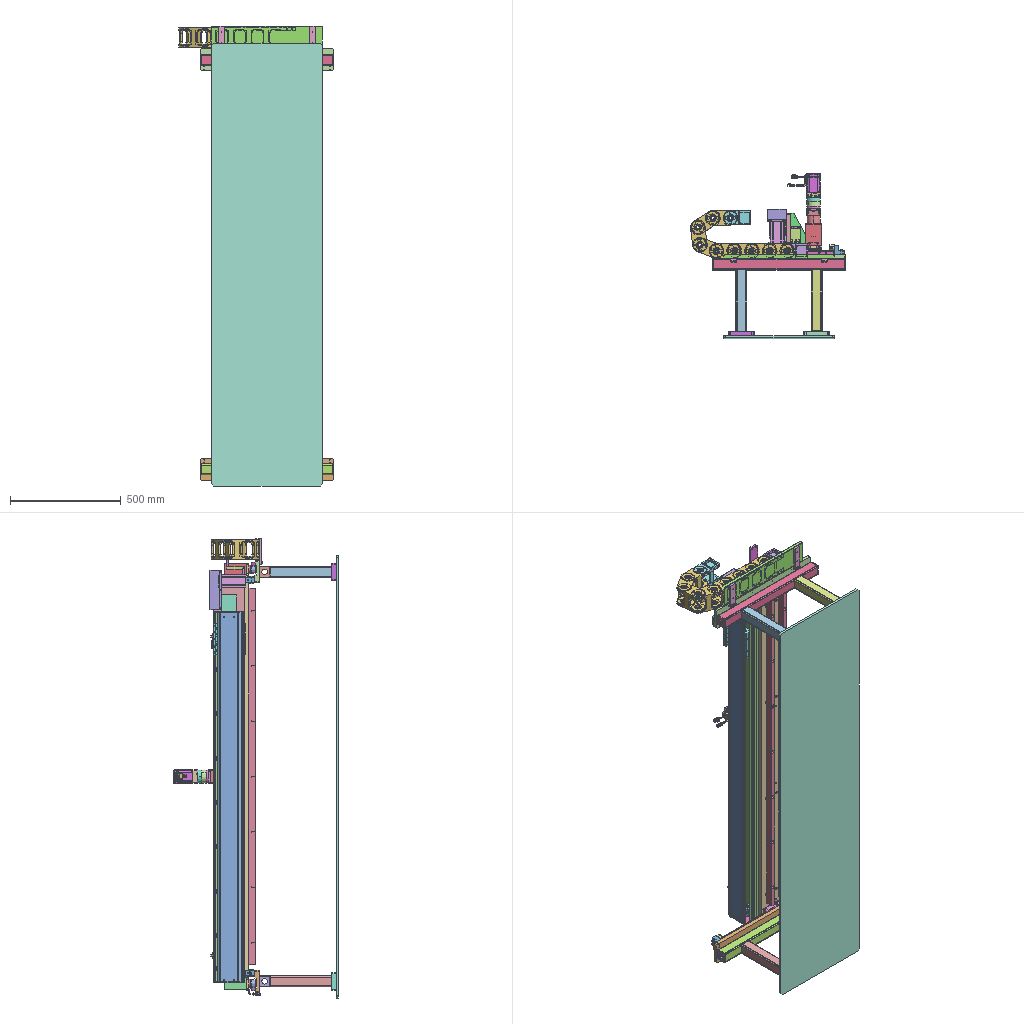Assembly | SolidWorks | 120 different items | 444 placed | box 699 x 745 x 2078 mm
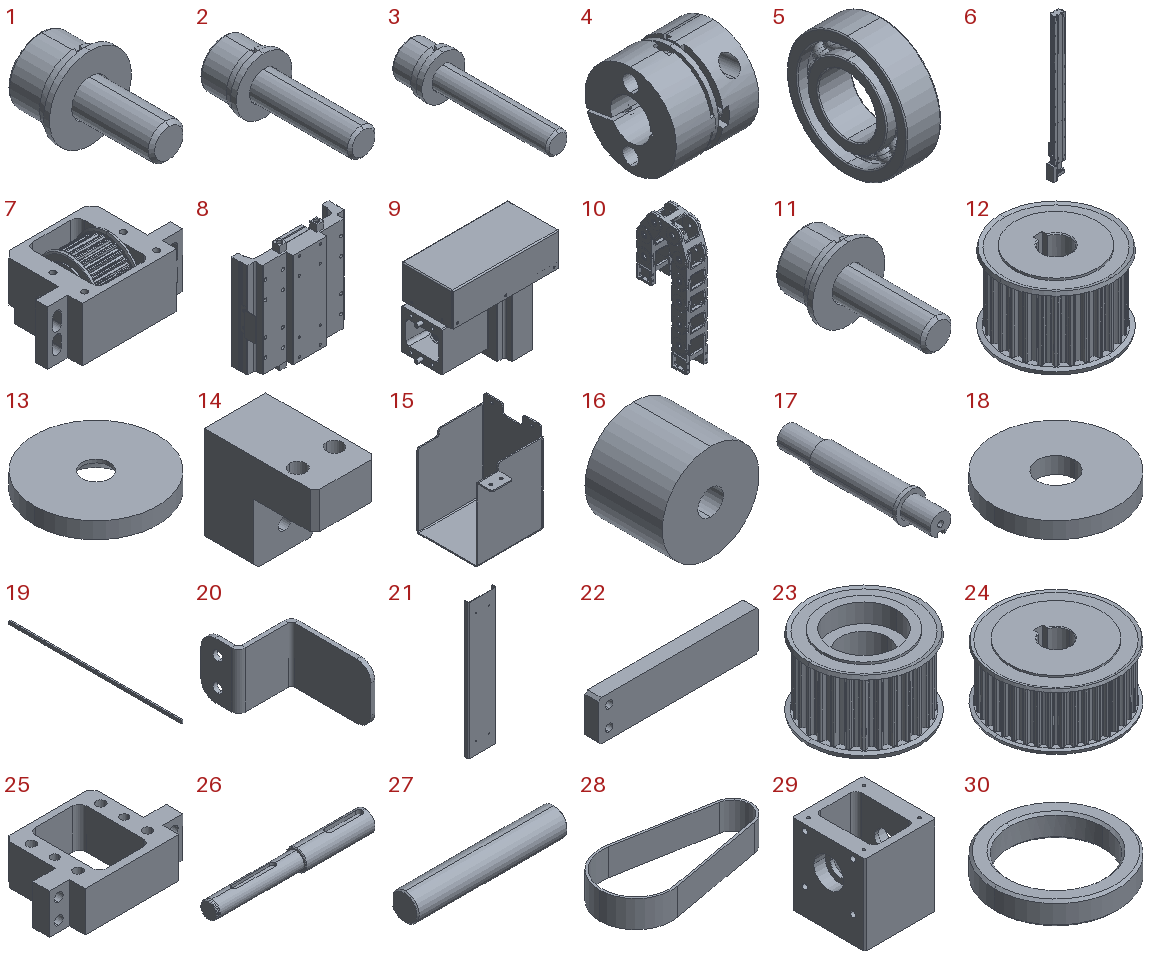Parts list (item | name | quantity | parent item | size | volume | features):
1 | (subassembly) | x2 | - | 7 x 11 x 7 mm | 152.048 mm3 | features RefAxis 1
2 | (subassembly) | x4 | - | 10 x 25 x 10 mm | 748.353 mm3 | features RefAxis 1
3 | (subassembly) | x12 | - | 12 x 41 x 12 mm | 1641 mm3 | features RefAxis 1
4 | (subassembly) | x2 | - | 29 x 32 x 32 mm | 15299 mm3 | -
5 | (subassembly) | x8 | - | 10 x 35 x 35 mm | 5427 mm3 | -
6 | (subassembly) | x1 | - | - | 6114333 mm3 | -
7 | (subassembly) | x1 | in 6 | 100 x 61 x 48 mm | 123898 mm3 | -
8 | (subassembly) | x2 | in 6 | 150 x 44 x 160 mm | 393138 mm3 | -
9 | (subassembly) | x1 | in 6 | 195.5 x 85 x 163 mm | 876200 mm3 | -
10 | (subassembly) | x1 | - | 93.598 x 215.392 x 529.568 mm | 1411050 mm3 | -
11 | (subassembly) | x4 | - | 7 x 13 x 7 mm | 166.185 mm3 | features RefAxis 1
12 | - | x1 | in 9 | 48 x 48 x 32 mm | 40101 mm3 | features BaseBody 1
13 | - | x2 | - | 15 x 15 x 2 mm | 317.309 mm3 | features Extrusion 1, HoleWzd 1
14 | - | x4 | - | 25 x 45 x 40 mm | 27816 mm3 | features Chamfer 2, HoleWzd 2, Extrusion 1, ICE 1
15 | - | x1 | - | 82.5 x 93.5 x 112 mm | 44800 mm3 | features EdgeFlange 2, HoleWzd 2, ICE 2, SMWeldBead 2, BreakCorner 1, FlatPattern 1, MoveFace 1, SMBaseFlange 1, SheetMetal 1
16 | - | x4 | - | 25 x 20 x 25 mm | 8476 mm3 | features Extrusion 1, HoleWzd 1
17 | - | x2 | - | 17 x 87.5 x 17 mm | 12724 mm3 | features ICE 3, HoleWzd 2, RefAxis 1, Revolution 1
18 | - | x4 | - | 15 x 15 x 2 mm | 321.621 mm3 | features Extrusion 1
19 | - | x2 | - | 18 x 1700 x 30 mm | 889358 mm3 | features Chamfer 1, Extrusion 1, HoleWzd 1
20 | - | x1 | - | 20.5 x 42 x 20 mm | 1726 mm3 | features BreakCorner 1, FlatPattern 1, HoleWzd 1, SMBaseFlange 1, SheetMetal 1
21 | - | x1 | - | 103 x 16.5 x 500 mm | 98465 mm3 | features BreakCorner 1, FlatPattern 1, HoleWzd 1, SMBaseFlange 1, SheetMetal 1
22 | - | x2 | - | 120 x 10 x 30 mm | 35369 mm3 | features HoleWzd 2, BreakCorner 1, FlatPattern 1, SMBaseFlange 1, SheetMetal 1
23 | - | x1 | in 7 | 48 x 48 x 32 mm | 29312 mm3 | features BaseBody 1
24 | - | x1 | in 9 | 67 x 67 x 32 mm | 86372 mm3 | features BaseBody 1
25 | - | x1 | in 6 | 100 x 63 x 30 mm | 67109 mm3 | features BaseBody 1
26 | - | x1 | in 9 | 114 x 15 x 15 mm | 15429 mm3 | features BaseBody 1
27 | - | x1 | in 7 | 66 x 12 x 12 mm | 7331 mm3 | features BaseBody 1
28 | - | x1 | in 9 | 140.79 x 66.7 x 25 mm | 16805 mm3 | features BaseBody 1
29 | - | x1 | in 9 | 66 x 68 x 75 mm | 164943 mm3 | features BaseBody 1
30 | - | x2 | in 7 | 16 x 16 x 3 mm | 250.27 mm3 | features BaseBody 1
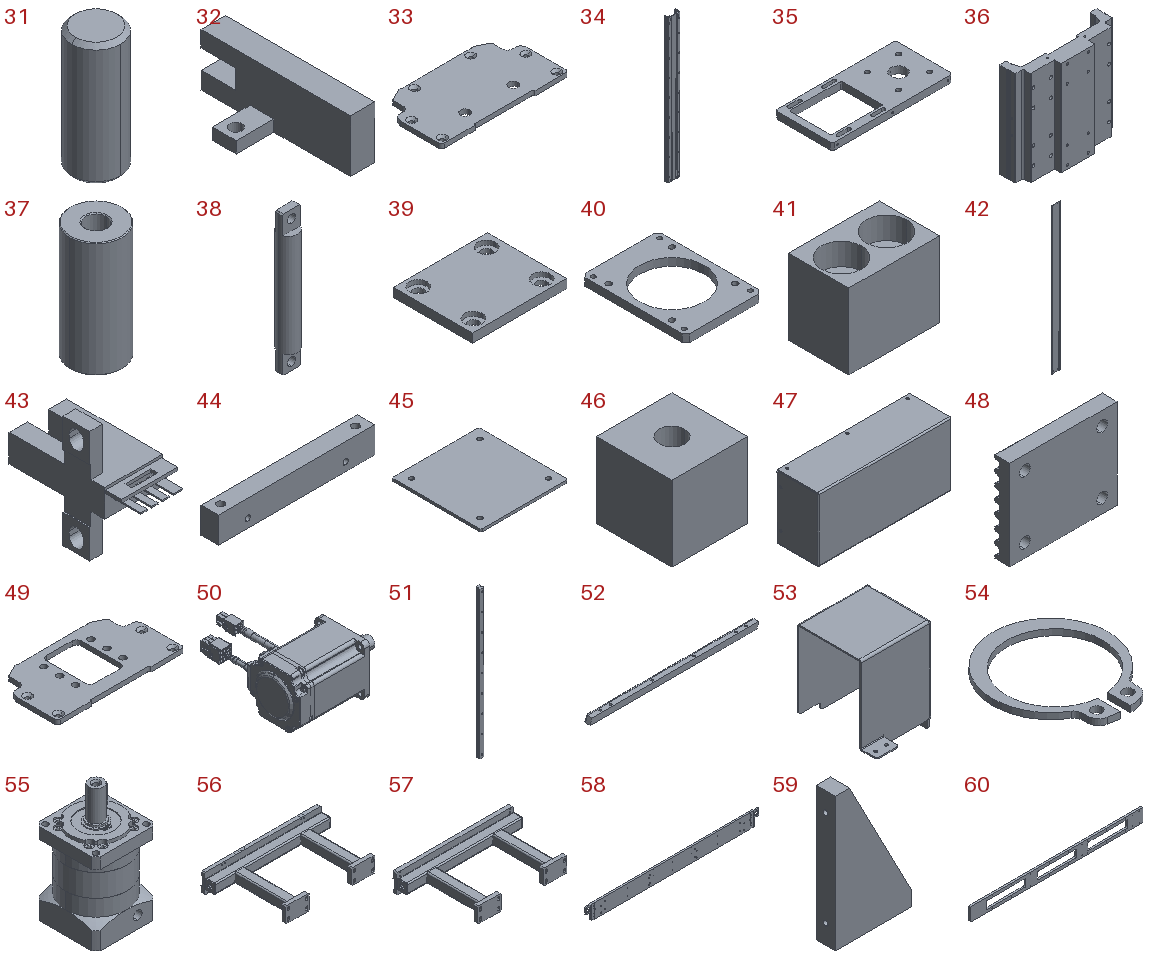31 | - | x2 | in 9 | 6 x 6 x 15 mm | 419.664 mm3 | features BaseBody 1
32 | - | x2 | in 6 | 26 x 39 x 13.7 mm | 3424 mm3 | features BaseBody 1
33 | - | x1 | in 6 | 140 x 76.005 x 5 mm | 46703 mm3 | features BaseBody 1
34 | - | x1 | in 6 | 140 x 53 x 1667 mm | 3998798 mm3 | features BaseBody 1
35 | - | x1 | in 9 | 175 x 83 x 10 mm | 88673 mm3 | features BaseBody 1
36 | - | x2 | in 8 | 144 x 44 x 140 mm | 348731 mm3 | features BaseBody 1
37 | - | x2 | in 8 | 20 x 20 x 44 mm | 11548 mm3 | features BaseBody 1
38 | - | x2 | in 8 | 8 x 8 x 60 mm | 2527 mm3 | features BaseBody 1
39 | - | x4 | in 8 | 43 x 36 x 4 mm | 5663 mm3 | features BaseBody 1
40 | - | x1 | in 9 | 60 x 82 x 6 mm | 17093 mm3 | features BaseBody 1
41 | - | x2 | in 6 | 18 x 12 x 15 mm | 2460 mm3 | features BaseBody 1
42 | - | x1 | in 6 | 109 x 8.5 x 1667 mm | 552829 mm3 | features BaseBody 1
43 | - | x3 | - | 13.7 x 28.4 x 26 mm | 1939 mm3 | features BaseBody 1
44 | - | x1 | in 6 | 72 x 8 x 12 mm | 6628 mm3 | features BaseBody 1
45 | - | x1 | in 9 | 66 x 68 x 2 mm | 8899 mm3 | features BaseBody 1
46 | - | x8 | in 8 | 10 x 10 x 10 mm | 827.255 mm3 | features BaseBody 1
47 | - | x1 | in 9 | 177 x 55 x 85 mm | 42380 mm3 | features BaseBody 1
48 | - | x4 | in 8 | 43 x 6 x 36 mm | 7398 mm3 | features BaseBody 1
49 | - | x1 | in 6 | 140 x 76.005 x 5 mm | 36774 mm3 | features BaseBody 1
50 | - | x1 | - | - | - | features RefSurface 19, BaseBody 5
51 | - | x1 | - | 15 x 15 x 500 mm | 91810 mm3 | features MirrorStock 1
52 | - | x1 | - | 506 x 17 x 17 mm | 126996 mm3 | features MirrorStock 1
53 | - | x1 | - | 82.5 x 93.5 x 112 mm | 44800 mm3 | features MirrorStock 1
54 | - | x8 | - | 18.95 x 21.754 x 1 mm | 100.896 mm3 | features Extrusion 1, Fillet 1
55 | - | x1 | - | 60 x 60 x 115 mm | 222679 mm3 | features BaseBody 7
56 | - | x1 | - | 600 x 368.308 x 100 mm | 1935248 mm3 | features HoleWzd 1, MirrorStock 1
57 | - | x1 | - | 600 x 368.308 x 100 mm | 1935957 mm3 | features HoleWzd 6, Chamfer 3, ICE 3, Cut 2, EndCap 1, MirrorPattern 1, WeldMemberFeat 1, WeldmentFeature 1
58 | - | x1 | - | 1924 x 20 x 160 mm | 5814736 mm3 | features HoleWzd 9, Cut 4, Chamfer 3, MirrorPattern 3, Fillet 2, Extrusion 1
59 | - | x4 | - | 80 x 20 x 140 mm | 141533 mm3 | features HoleWzd 2, Extrusion 1, ICE 1
60 | - | x1 | - | 1814 x 20 x 140 mm | 3064882 mm3 | features HoleWzd 3, Chamfer 1, Cut 1, Extrusion 1, Fillet 1
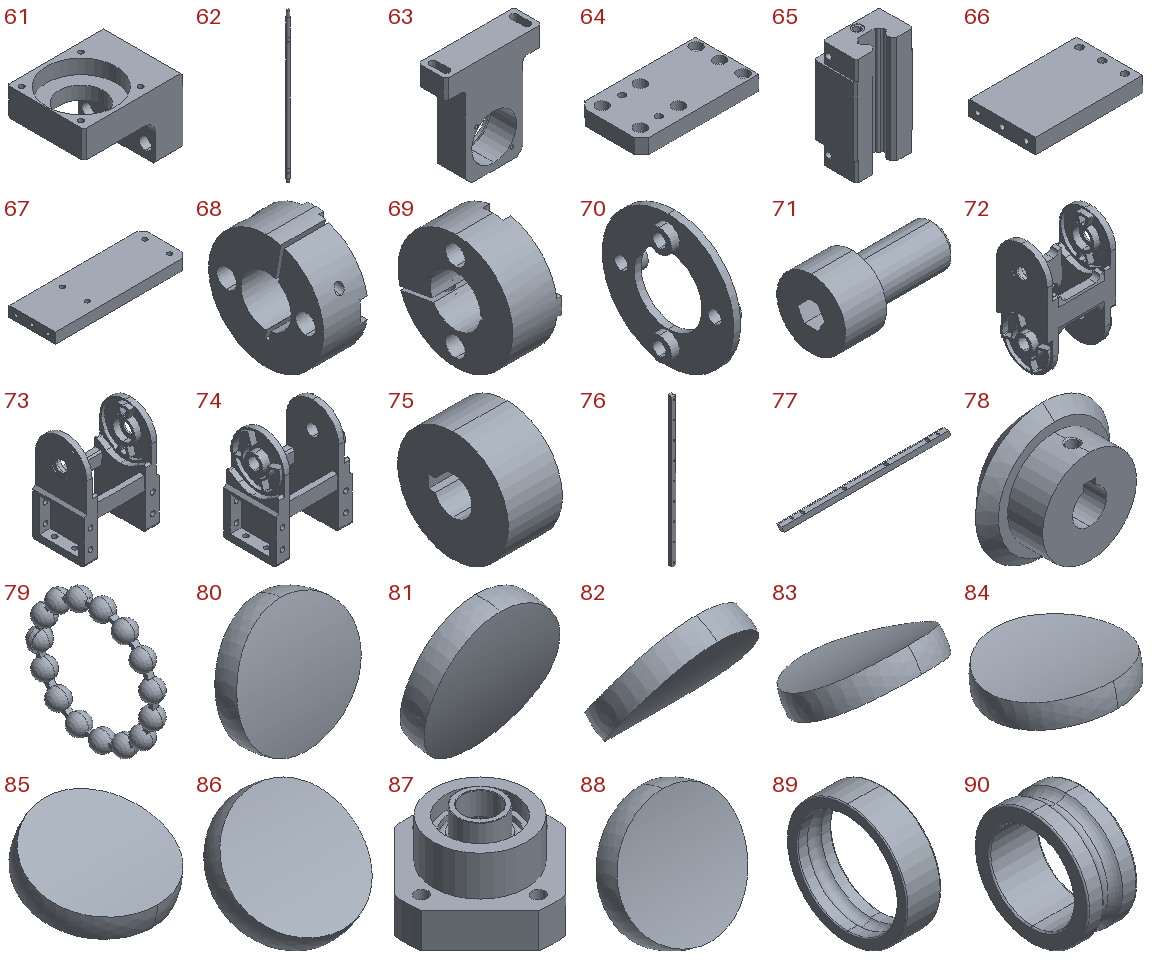61 | - | x2 | - | 90 x 70 x 60 mm | 158860 mm3 | features Cut 2, HoleWzd 2, Chamfer 1, Extrusion 1, Fillet 1
62 | - | x2 | - | 17 x 17 x 847.55 mm | 187223 mm3 | features ICE 7, Cut 1, Extrusion 1, HoleWzd 1, MoveFace 1
63 | - | x4 | - | 75 x 22 x 80 mm | 65225 mm3 | features ICE 3, Chamfer 2, HoleWzd 2, CirPattern 1, Extrusion 1, Fillet 1
64 | - | x1 | - | 80 x 43.6 x 10 mm | 31034 mm3 | features HoleWzd 3, Chamfer 1, Extrusion 1
65 | - | x4 | - | 34 x 23.7 x 61.4 mm | 36561 mm3 | features BaseBody 1
66 | - | x1 | - | 71 x 43.6 x 10 mm | 29737 mm3 | features HoleWzd 2, Extrusion 1
67 | - | x1 | - | 126 x 43.6 x 10 mm | 53864 mm3 | features HoleWzd 2, Chamfer 1, Extrusion 1
68 | - | x2 | in 4 | 13.7 x 32 x 32 mm | 6947 mm3 | features BaseBody 1
69 | - | x2 | in 4 | 13.7 x 32 x 32 mm | 6989 mm3 | features BaseBody 1
70 | - | x2 | in 4 | 5.6 x 31 x 31 mm | 974.208 mm3 | features BaseBody 1
71 | - | x8 | in 4 | 9 x 5 x 5 mm | 97.086 mm3 | features BaseBody 1
72 | - | x8 | in 10 | 89 x 65.39 x 145.39 mm | 145575 mm3 | features BaseBody 1
73 | - | x1 | in 10 | 93.538 x 64.35 x 124.74 mm | 121596 mm3 | features BaseBody 1
74 | - | x1 | in 10 | 93.598 x 64.35 x 124.74 mm | 124855 mm3 | features BaseBody 1
75 | - | x2 | - | 17 x 34.83 x 34.83 mm | 14145 mm3 | features BaseBody 1, ICE 1
76 | - | x1 | - | 15 x 15 x 500 mm | 91810 mm3 | features BaseBody 1, HoleWzd 1, ICE 1, MoveFace 1
77 | - | x1 | - | 506 x 17 x 17 mm | 126996 mm3 | features BaseBody 1
78 | - | x4 | - | 47.12 x 22.819 x 47.12 mm | 20583 mm3 | features 3DProfileFeature 1, BaseBody 1
79 | - | x8 | in 5 | 4.95 x 30.216 x 30.358 mm | 737.087 mm3 | features BaseBody 1
80 | - | x8 | in 5 | 4.95 x 1.888 x 4.932 mm | 17.147 mm3 | features BaseBody 1
81 | - | x8 | in 5 | 4.95 x 1.888 x 4.932 mm | 17.147 mm3 | features BaseBody 1
82 | - | x8 | in 5 | 4.95 x 3.576 x 4.449 mm | 17.147 mm3 | features BaseBody 1
83 | - | x8 | in 5 | 4.95 x 4.646 x 3.202 mm | 17.147 mm3 | features BaseBody 1
84 | - | x8 | in 5 | 4.95 x 4.95 x 1.444 mm | 17.147 mm3 | features BaseBody 1
85 | - | x8 | in 5 | 4.95 x 4.886 x 2.353 mm | 17.147 mm3 | features BaseBody 1
86 | - | x8 | in 5 | 4.95 x 4.203 x 3.911 mm | 17.147 mm3 | features BaseBody 1
87 | - | x2 | - | 63 x 63 x 46 mm | 51941 mm3 | features BaseBody 1
88 | - | x8 | in 5 | 4.95 x 2.793 x 4.793 mm | 17.147 mm3 | features BaseBody 1
89 | - | x8 | in 5 | 10 x 35 x 35 mm | 2757 mm3 | features BaseBody 1
90 | - | x8 | in 5 | 10 x 23 x 23 mm | 1693 mm3 | features BaseBody 1
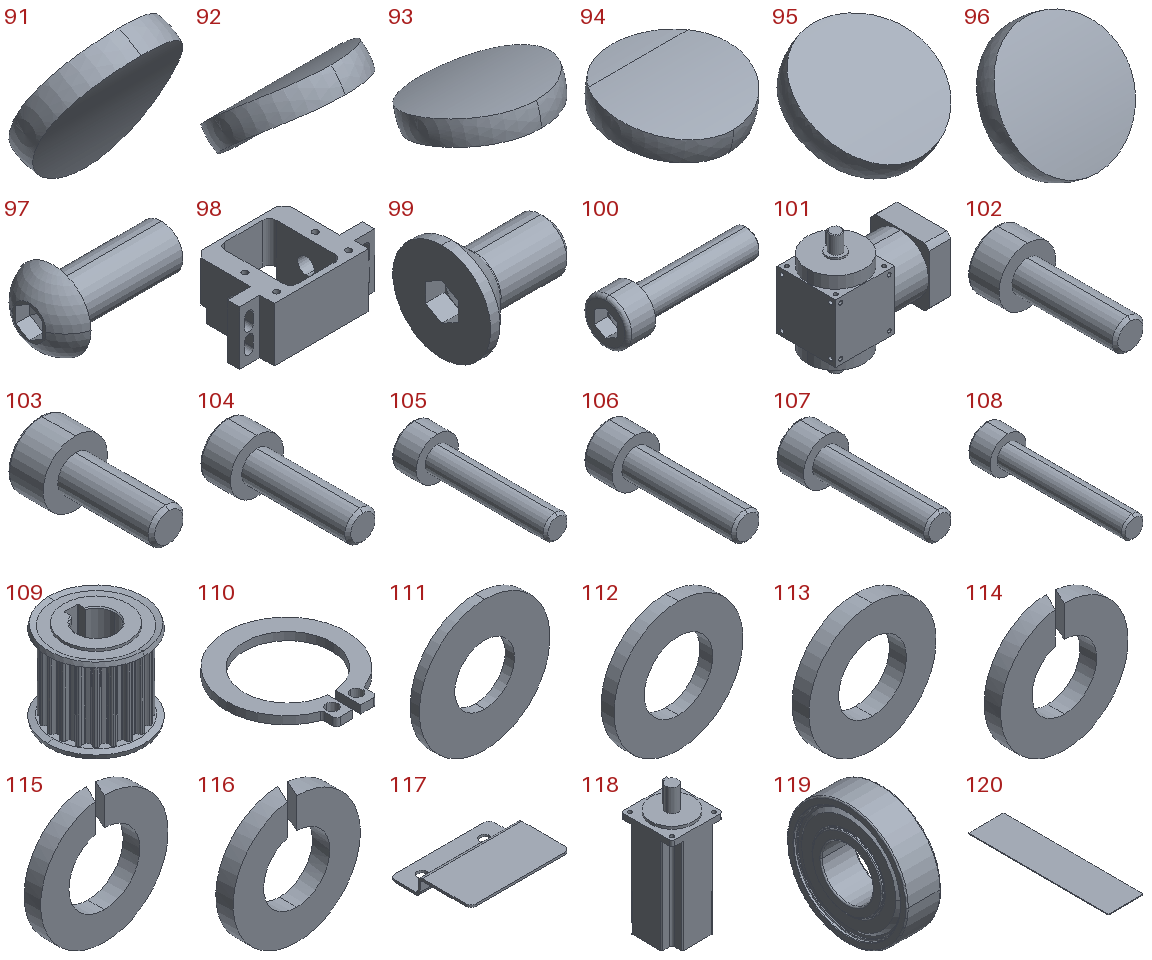91 | - | x8 | in 5 | 4.95 x 2.793 x 4.793 mm | 17.147 mm3 | features BaseBody 1
92 | - | x8 | in 5 | 4.95 x 4.203 x 3.911 mm | 17.147 mm3 | features BaseBody 1
93 | - | x8 | in 5 | 4.95 x 4.886 x 2.353 mm | 17.147 mm3 | features BaseBody 1
94 | - | x8 | in 5 | 4.95 x 4.95 x 1.444 mm | 17.148 mm3 | features BaseBody 1
95 | - | x8 | in 5 | 4.95 x 4.646 x 3.202 mm | 17.147 mm3 | features BaseBody 1
96 | - | x8 | in 5 | 4.95 x 3.576 x 4.449 mm | 17.147 mm3 | features BaseBody 1
97 | - | x8 | - | 48.8 x 28 x 28 mm | 11109 mm3 | features Cut 2, RevCut 2, Boss 1, Extrusion 1, Fillet 1, LPattern 1
98 | - | x1 | in 7 | 100 x 61 x 40 mm | 80408 mm3 | features BaseBody 1
99 | - | x2 | - | 8 x 7.53 x 7.53 mm | 138.584 mm3 | features RevCut 3, Chamfer 1, Cut 1, Fillet 1, LPattern 1, Revolution 1
100 | - | x4 | - | 31 x 10 x 10 mm | 1099 mm3 | features Fillet 2, RevCut 2, Boss 1, Chamfer 1, Cut 1, Extrusion 1, LPattern 1
101 | - | x1 | - | 128 x 65 x 134 mm | 554755 mm3 | features BaseBody 1
102 | - | x4 | in 11 | 5.5 x 13 x 5.5 mm | 134.154 mm3 | features ICE 2, Chamfer 1, Extrusion 1, Fillet 1, RefAxis 1
103 | - | x2 | in 1 | 5.5 x 11 x 5.5 mm | 120.016 mm3 | features ICE 2, Chamfer 1, Extrusion 1, Fillet 1, RefAxis 1
104 | - | x5 | - | 7 x 18 x 7 mm | 312.463 mm3 | features ICE 2, Chamfer 1, Extrusion 1, Fillet 1, RefAxis 1
105 | - | x18 | - | 7 x 24 x 7 mm | 387.861 mm3 | features ICE 2, Chamfer 1, Extrusion 1, Fillet 1, RefAxis 1
106 | - | x12 | in 2 | 8.5 x 25 x 8.5 mm | 639.095 mm3 | features ICE 2, Chamfer 1, Extrusion 1, Fillet 1, RefAxis 1
107 | - | x4 | - | 10 x 31 x 10 mm | 1108 mm3 | features ICE 2, Chamfer 1, Extrusion 1, Fillet 1, RefAxis 1
108 | - | x12 | in 3 | 10 x 41 x 10 mm | 1390 mm3 | features ICE 2, Chamfer 1, Extrusion 1, Fillet 1, RefAxis 1
109 | - | x1 | in 9 | 36 x 36 x 32 mm | 16182 mm3 | features BaseBody 1
110 | - | x1 | in 9 | 15.3 x 16.6 x 1 mm | 87.791 mm3 | features BaseBody 1
111 | - | x6 | in 1, 11 | 7 x 0.5 x 7 mm | 15.221 mm3 | features Extrusion 1, RefAxis 1
112 | - | x4 | in 2 | 10 x 1 x 10 mm | 56.478 mm3 | features Extrusion 1, RefAxis 1
113 | - | x12 | in 3 | 12 x 1.6 x 12 mm | 129.484 mm3 | features Extrusion 1, RefAxis 1
114 | - | x6 | in 1, 11 | 6.1 x 0.8 x 6.1 mm | 16.81 mm3 | features Extrusion 1, ICE 1, RefAxis 1
115 | - | x4 | in 2 | 9.15 x 1.2 x 9.15 mm | 52.779 mm3 | features Extrusion 1, ICE 1, RefAxis 1
116 | - | x12 | in 3 | 11.7 x 1.6 x 11.7 mm | 121.294 mm3 | features Extrusion 1, ICE 1, RefAxis 1
117 | - | x2 | in 8 | 35 x 28.6 x 6 mm | 900.941 mm3 | features BaseBody 1
118 | - | x1 | in 9 | 60 x 60 x 148 mm | 371098 mm3 | features BaseBody 1
119 | - | x4 | in 7, 9 | 8 x 28 x 28 mm | 3240 mm3 | features BaseBody 1
120 | - | x1 | - | 500 x 2000 x 10 mm | 9998000 mm3 | features Chamfer 1, Extrusion 1
Mates (type | each side: item.copy, entity, surface, feature):
In the top assembly
Coincident | 57.1 face plane Gb/6728-1986方形空心型钢 50 X 50 X 3(1) | 56.1 face plane
Coincident | 57.1 face plane Boss-Extrude 2 | 56.1 face plane
DistanceDim | 57.1 face plane Gb/6728-1986方形空心型钢 50 X 50 X 3(1) | 56.1 face plane
Coincident | 57.1 plane | assembly plane | 2 times
Symmetric | 57.1 face plane Gb/6728-1986方形空心型钢 50 X 50 X 3(1) | 56.1 face plane | assembly plane
Width | 76.1 face plane 输入1 | 76.1 face plane 输入1 | 57.1 face plane Boss-Extrude 2 | 57.1 face plane Boss-Extrude 2
DistanceDim | 76.1 plane | 57.1 face plane Boss-Extrude 2
Coincident | 65.1 face plane 输入1 | 76.1 face plane 输入1
Width | 65.1 face plane 输入1 | 65.1 face plane 输入1 | 76.1 face plane 输入1 | 76.1 face plane 输入1
Coincident | 76.1 face plane 输入1 | 65.2 face plane 输入1
Coincident | 65.1 face plane 输入1 | 65.2 face plane 输入1
DistanceDim | 65.2 face plane 输入1 | 65.1 face plane 输入1
Width | 65.2 face plane 输入1 | 65.1 face plane 输入1 | 58.1 face plane Boss-Extrude 1 | 58.1 face plane Boss-Extrude 1
Width | 57.1 face plane Gb/6728-1986方形空心型钢 50 X 50 X 3(1) | 56.1 face plane | 58.1 face plane Boss-Extrude 1 | 58.1 face plane Boss-Extrude 1
Width | 57.1 face plane Boss-Extrude 2 | 57.1 face plane Boss-Extrude 2 | 77.1 plane | 77.1 plane
Coincident | 58.1 face plane Boss-Extrude 1 | 60.1 face plane Boss-Extrude 1 | 2 times
Width | 60.1 face plane Boss-Extrude 1 | 60.1 face plane Boss-Extrude 1 | 58.1 face plane Boss-Extrude 1 | 58.1 face plane Boss-Extrude 1
Coincident | 60.1 face plane Boss-Extrude 1 | 34.1 face plane 输入1 | 2 times
Width | 60.1 face plane Boss-Extrude 1 | 60.1 face plane Boss-Extrude 1 | 33.1 face plane 输入1 | 47.1 face plane 输入1
Coincident | 101.1 face plane 输入1 | 55.1 face plane PRF60 Upper蓋版_D1-70 D2-5.5 D3-14 D4-17 D5-50 L1-30 L2-35 L3-3 A1-60 S1-3 S2-20 S3-5 S4-18 B-5 H-16 C-M5 标准-1-solid1
Concentric | 101.1 face cylinder 输入1 | 55.1 face cylinder PRF60 Upper蓋版_D1-70 D2-5.5 D3-14 D4-17 D5-50 L1-30 L2-35 L3-3 A1-60 S1-3 S2-20 S3-5 S4-18 B-5 H-16 C-M5 标准-1-solid1
Concentric | 50.1 face cylinder DEFAULT-1/DEFAULT-1-surface1 | 55.1 face cylinder PRF60 Lower蓋版_D6-60 D7-14 标准-1-solid1
Parallel | 50.1 face plane DEFAULT-1/DEFAULT-1-surface2 | 55.1 face plane PRF60-連接Plate-标准_D8-50 D9-70 D10-M10 L4-22 L6-32(22+10) L7-4 A2-60 R-39.5 标准-1-solid1
Coincident | 50.1 face plane DEFAULT-1/DEFAULT-1-surface2 | 55.1 face plane PRF60-連接Plate-标准_D8-50 D9-70 D10-M10 L4-22 L6-32(22+10) L7-4 A2-60 R-39.5 标准-1-solid1
Parallel | 101.1 face plane 输入1 | 55.1 face plane PRF60 Upper蓋版_D1-70 D2-5.5 D3-14 D4-17 D5-50 L1-30 L2-35 L3-3 A1-60 S1-3 S2-20 S3-5 S4-18 B-5 H-16 C-M5 标准-1-solid1
Parallel | 60.1 face plane Boss-Extrude 1 | 101.1 face plane 输入1
Width | 60.1 face plane Boss-Extrude 1 | 60.1 face plane Boss-Extrude 1 | 101.1 face plane 输入1 | 101.1 face plane 输入1
Coincident | 58.1 face plane Boss-Extrude 1 | 61.1 face plane Boss-Extrude 1
Width | 61.1 face plane Boss-Extrude 1 | 61.1 face plane Boss-Extrude 1 | 101.1 face plane 输入1 | 101.1 face plane 输入1
Coincident | 101.1 face plane 输入1 | 61.1 face plane Boss-Extrude 1
Coincident | 58.1 face plane Boss-Extrude 1 | 61.2 face plane Boss-Extrude 1
Coincident | 61.1 face plane Boss-Extrude 1 | 61.2 face plane Boss-Extrude 1
Coincident | 101.1 face plane 输入1 | 61.2 face plane Boss-Extrude 1
Concentric | 101.1 face cylinder 输入1 | 69.1 face cylinder 输入1
Concentric | 69.1 face cylinder 输入1 | 62.1 face cylinder Boss-Extrude 1
Coincident | 101.1 face plane 输入1 | 69.1 face plane 输入1
Coincident | 68.1 face plane 输入1 | 62.1 face plane Boss-Extrude 1
Concentric | 62.1 face cylinder Boss-Extrude 2 | 90.1 face cylinder 输入1
Concentric | 62.1 face cylinder Boss-Extrude 2 | 63.1 face cylinder Cut-Extrude 3
Parallel | 58.1 face plane Boss-Extrude 1 | 63.1 face plane Boss-Extrude 1
Coincident | 89.1 face plane 输入1 | 63.1 face plane Boss-Extrude 3
Concentric | 62.1 face cylinder Boss-Extrude 2 | 90.2 face cylinder 输入1
Coincident | 63.1 face plane Boss-Extrude 1 | 89.2 face plane 输入1
Coincident | 63.2 face plane Boss-Extrude 1 | 89.3 face plane 输入1
Concentric | 63.2 face cylinder Cut-Extrude 3 | 90.3 face cylinder 输入1
Concentric | 90.4 face cylinder 输入1 | 90.3 face cylinder 输入1
Coincident | 58.1 face plane Boss-Extrude 1 | 63.2 face plane Boss-Extrude 1
Coincident | 89.4 face plane 输入1 | 89.3 face plane 输入1
Coincident | 63.1 face plane Boss-Extrude 1 | 63.2 face plane Boss-Extrude 1
DistanceDim | 63.1 face plane Boss-Extrude 1 | 58.1 face plane Boss-Extrude 1
Coincident | 58.1 face plane Boss-Extrude 1 | 63.1 face plane Boss-Extrude 2
Concentric | 62.1 face cylinder Cut-Extrude 1 | 78.1 face cylinder 输入1
Coincident | 62.1 face plane Boss-Extrude 2 | 78.1 face plane 输入1
Coincident | 78.1 select_type:25 | 78.2 select_type:25
Parallel | 58.1 face plane Boss-Extrude 1 | 78.2 face plane 输入1
GearDim | 78.1 edge | 78.2 edge
Concentric | 101.1 face cylinder 输入1 | 61.2 face cylinder Cut-Extrude 2
Concentric | 78.2 face cylinder 输入1 | 17.1 face cylinder Revolve 1
Coincident | 78.2 face plane 输入1 | 17.1 face plane Revolve 1
Concentric | 17.1 face cylinder Revolve 1 | 87.1 face cylinder 输入1
Parallel | 58.1 face plane Boss-Extrude 1 | 87.1 face plane 输入1
Coincident | 58.1 face plane Cut-Extrude 1 | 87.1 face plane 输入1
Coincident | 57.1 face plane Boss-Extrude 2 | 76.1 face plane 输入1
Coincident | 57.1 face plane Cut-Extrude 2 | 77.1 face plane 输入1
DistanceDim | 17.1 axis | 77.1 face plane 输入1
Concentric | 17.1 face cylinder Boss-Extrude 1 | 75.1 face cylinder 输入1 | 2 times
Coincident | 17.1 face plane Revolve 1 | 75.1 face plane 输入1
DistanceDim | 58.1 face plane Boss-Extrude 1 | 65.1 face plane 输入1
Coincident | 62.1 face plane Cut-Extrude 11 | 78.1 face plane 输入1
Coincident | 78.2 face plane 输入1 | 17.1 face plane Cut-Extrude 1
Coincident | 58.1 face plane Boss-Extrude 1 | 59.1 face plane Boss-Extrude 1
Coincident | 59.1 face plane Boss-Extrude 1 | 60.1 face plane Boss-Extrude 1
Coincident | 58.1 face plane Boss-Extrude 1 | 59.2 face plane Boss-Extrude 1
Coincident | 60.1 face plane Boss-Extrude 1 | 59.2 face plane Boss-Extrude 1
DistanceDim | 60.1 face plane Boss-Extrude 1 | 59.1 face plane Boss-Extrude 1
DistanceDim | 59.2 face plane Boss-Extrude 1 | 60.1 face plane Boss-Extrude 1
Concentric | 17.1 face cylinder M4 Tapped Hole 2 | 18.1 face cylinder Boss-Extrude 1
Concentric | 18.1 face cylinder Boss-Extrude 1 | 100.1 face cylinder BaseBody
Coincident | 18.1 face plane Boss-Extrude 1 | 100.1 face plane BaseHead
Concentric | 75.1 face cylinder 输入1 | 13.1 face cylinder Boss-Extrude 1
Coincident | 17.1 face plane Boss-Extrude 1 | 13.1 face plane Boss-Extrude 1
Concentric | 13.1 face cylinder M3 开槽沉头木Screw的锥形沉头Hole 1 | 99.1 face cylinder Base
DistanceDim | 63.2 face plane Boss-Extrude 1 | 58.1 face plane Cut-Extrude 1
Width | 19.1 face plane Boss-Extrude 1 | 19.1 face plane Boss-Extrude 1 | 58.1 face plane Cut-Extrude 1 | 58.1 face plane Mirror 1
DistanceDim | 58.1 face plane Boss-Extrude 1 | 19.1 face plane Boss-Extrude 1
Coincident | 78.2 face plane 输入1 | 18.1 face plane Boss-Extrude 1
Coincident | 13.1 face cone M3 开槽沉头木Screw的锥形沉头Hole 1 | 99.1 face cone Base
Coincident | 58.1 face plane Boss-Extrude 1 | 19.1 face plane Boss-Extrude 1
Coincident | 58.1 face plane Boss-Extrude 1 | 19.2 face plane Boss-Extrude 1
Width | 19.1 face plane Boss-Extrude 1 | 19.2 face plane Boss-Extrude 1 | 58.1 face plane Boss-Extrude 1 | 58.1 face plane Boss-Extrude 1
Coincident | 19.1 face plane Boss-Extrude 1 | 19.2 face plane Boss-Extrude 1
Coincident | 57.1 face plane Boss-Extrude 2 | 14.1 face plane Boss-Extrude 1
Width | 14.1 face plane Boss-Extrude 1 | 14.1 face plane Boss-Extrude 1 | 76.1 face plane 输入1 | 76.1 face plane 输入1
Coincident | 76.1 face plane 输入1 | 14.1 face plane Boss-Extrude 1
Concentric | 14.1 face cylinder M6 Tapped Hole 1 | 16.1 face cylinder M6 六角圆柱头Screw的柱形沉头Hole 1
Coincident | 14.1 face plane Boss-Extrude 1 | 16.1 face plane Boss-Extrude 1
Coincident | 57.1 face plane Boss-Extrude 2 | 43.1 face plane 输入1
Width | 57.1 face plane Cut-Extrude 2 | 57.1 face plane Boss-Extrude 2 | 43.1 face plane 输入1 | 43.1 face plane 输入1
Coincident | 57.1 face plane Boss-Extrude 2 | 43.2 face plane 输入1
Width | 57.1 face plane Cut-Extrude 2 | 57.1 face plane Boss-Extrude 2 | 43.2 face plane 输入1 | 43.2 face plane 输入1
DistanceDim | 57.1 face plane Boss-Extrude 2 | 43.2 face plane 输入1
Coincident | 43.2 face plane 输入1 | 43.3 face plane 输入1 | 2 times
DistanceDim | 43.3 face plane 输入1 | 43.2 face plane 输入1
Coincident | 58.1 face plane Boss-Extrude 1 | 20.1 face plane Base-Flange 1
Width | 58.1 face plane Boss-Extrude 1 | 58.1 face plane Cut-Extrude 5 | 20.1 face plane Base-Flange 1 | 20.1 face plane Base-Flange 1
Coincident | 58.1 face plane Cut-Extrude 1 | 20.1 face plane Base-Flange 1
Concentric | 62.1 face cylinder M4 Tapped Hole 1 | 18.2 face cylinder Boss-Extrude 1
Coincident | 62.1 face plane Cut-Extrude 2 | 18.2 face plane Boss-Extrude 1
Concentric | 62.1 face cylinder M4 Tapped Hole 1 | 100.2 face cylinder BaseBody
Coincident | 100.2 face plane BaseHead | 18.2 face plane Boss-Extrude 1
Concentric | 63.2 face cylinder M3 Tapped Hole 1 | 97.1 face cylinder BaseBody
Coincident | 63.2 face plane Boss-Extrude 1 | 97.1 face plane BaseHead
Concentric | 63.2 face cylinder CirPattern 1 | 97.2 face cylinder BaseBody
Coincident | 63.2 face plane Boss-Extrude 1 | 97.2 face plane BaseHead
Concentric | 63.1 face cylinder M3 Tapped Hole 1 | 97.3 face cylinder BaseBody
Coincident | 63.1 face plane Boss-Extrude 1 | 97.3 face plane BaseHead
Concentric | 63.1 face cylinder CirPattern 1 | 97.4 face cylinder BaseBody
Coincident | 63.1 face plane Boss-Extrude 1 | 97.4 face plane BaseHead
Concentric | 62.1 face cylinder Cut-Extrude 15 | 54.1 face cylinder Boss-Extrude 1
Coincident | 90.3 face plane 输入1 | 54.1 face plane Boss-Extrude 1
Concentric | 62.1 face cylinder Cut-Extrude 14 | 54.2 face cylinder Boss-Extrude 1
Coincident | 90.4 face plane 输入1 | 54.2 face plane Boss-Extrude 1
Concentric | 62.1 face cylinder Cut-Extrude 13 | 54.3 face cylinder Boss-Extrude 1
Coincident | 90.1 face plane 输入1 | 54.3 face plane Boss-Extrude 1
Concentric | 62.1 face cylinder Cut-Extrude 12 | 54.4 face cylinder Boss-Extrude 1
Coincident | 90.2 face plane 输入1 | 54.4 face plane Boss-Extrude 1
Width | 21.1 face plane Base-Flange 1 | 21.1 face plane Base-Flange 1 | 56.1 face plane | 56.1 face plane
Coincident | 56.1 face plane | 21.1 face plane Base-Flange 1 | 2 times
Coincident | 56.1 face plane | 22.1 face plane Base-Flange 1
Coincident | 21.1 face plane Base-Flange 1 | 22.1 face plane Base-Flange 1
Coincident | 21.1 face plane Base-Flange 1 | 72.1 face plane 输入1
Width | 21.1 face plane Base-Flange 1 | 21.1 face plane Base-Flange 1 | 74.1 face plane 输入1 | 74.1 face plane 输入1
DistanceDim | 74.1 face plane 输入1 | 21.1 face plane Base-Flange 1
Coincident | 56.1 face plane | 22.2 face plane Base-Flange 1
Coincident | 21.1 face plane Base-Flange 1 | 22.2 face plane Base-Flange 1
Width | 21.1 face plane Base-Flange 1 | 21.1 face plane Base-Flange 1 | 22.2 face plane Base-Flange 1 | 22.1 face plane Base-Flange 1
LimitDistanceDim | 58.1 face plane Boss-Extrude 1 | 16.2 face plane Boss-Extrude 1
Coincident | 58.1 face plane Cut-Extrude 1 | 15.1 face plane Edge-Flange 1
Width | 87.1 face plane 输入1 | 87.1 face plane 输入1 | 15.1 face plane Edge-Flange 1 | 15.1 face plane Edge-Flange 1
Coincident | 58.1 face plane Boss-Extrude 1 | 15.1 face plane Edge-Flange 1
Coincident | 58.1 face plane Boss-Extrude 1 | 64.1 face plane Boss-Extrude 1
Symmetric | 65.3 plane | 64.1 face plane Boss-Extrude 1 | 64.1 face plane Boss-Extrude 1
DistanceDim | 64.1 face plane Boss-Extrude 1 | 58.1 face plane Mirror 1
Coincident | 64.1 face plane Boss-Extrude 1 | 66.1 face plane Boss-Extrude 1 | 4 times
Coincident | 66.1 face plane Boss-Extrude 1 | 67.1 face plane Boss-Extrude 1 | 3 times
DistanceDim | 22.2 face plane Base-Flange 1 | 21.1 face plane Base-Flange 1
Coincident | 57.1 face plane Boss-Extrude 3 | 120.1 face plane Boss-Extrude 1
Width | 120.1 face plane Boss-Extrude 1 | 120.1 face plane Boss-Extrude 1 | 57.1 face plane Boss-Extrude 3 | 57.1 face plane Boss-Extrude 3
Width | 120.1 face plane Boss-Extrude 1 | 120.1 face plane Boss-Extrude 1 | 57.1 face plane Boss-Extrude 3 | 56.1 face plane
Coincident | 77.1 face plane 输入1 | 106.1 plane
Concentric | 57.1 face cylinder M5 Tapped Hole 1 | 106.1 axis
Coincident | 77.1 face plane 输入1 | 106.2 plane
Concentric | 57.1 face cylinder M5 Tapped Hole 1 | 106.2 axis
Coincident | 77.1 face plane 输入1 | 106.3 plane
Concentric | 57.1 face cylinder M5 Tapped Hole 1 | 106.3 axis
Coincident | 77.1 face plane 输入1 | 106.4 plane
Concentric | 57.1 face cylinder M5 Tapped Hole 1 | 106.4 axis
Coincident | 76.1 face plane M4 六角圆柱头Screw的柱形沉头Hole 1 | 105.1 plane
Concentric | 57.1 face cylinder M4 Tapped Hole 1 | 105.1 axis
Coincident | 76.1 face plane M4 六角圆柱头Screw的柱形沉头Hole 1 | 105.2 plane
Concentric | 57.1 face cylinder M4 Tapped Hole 1 | 105.2 axis
Coincident | 76.1 face plane M4 六角圆柱头Screw的柱形沉头Hole 1 | 105.3 plane
Concentric | 57.1 face cylinder M4 Tapped Hole 1 | 105.3 axis
Coincident | 76.1 face plane M4 六角圆柱头Screw的柱形沉头Hole 1 | 105.4 plane
Concentric | 57.1 face cylinder M4 Tapped Hole 1 | 105.4 axis
Coincident | 76.1 face plane M4 六角圆柱头Screw的柱形沉头Hole 1 | 105.5 plane
Concentric | 57.1 face cylinder M4 Tapped Hole 1 | 105.5 axis
Coincident | 76.1 face plane M4 六角圆柱头Screw的柱形沉头Hole 1 | 105.6 plane
Concentric | 57.1 face cylinder M4 Tapped Hole 1 | 105.6 axis
Coincident | 76.1 face plane M4 六角圆柱头Screw的柱形沉头Hole 1 | 105.7 plane
Concentric | 57.1 face cylinder M4 Tapped Hole 1 | 105.7 axis
Coincident | 76.1 face plane M4 六角圆柱头Screw的柱形沉头Hole 1 | 105.8 plane
Concentric | 57.1 face cylinder M4 Tapped Hole 1 | 105.8 axis
Coincident | 76.1 face plane M4 六角圆柱头Screw的柱形沉头Hole 1 | 105.9 plane
Concentric | 57.1 face cylinder M4 Tapped Hole 1 | 105.9 axis
Coincident | 16.1 face plane M6 六角圆柱头Screw的柱形沉头Hole 1 | 107.1 plane
Concentric | 14.1 face cylinder M6 Tapped Hole 1 | 107.1 axis
Coincident | 16.3 face plane M6 六角圆柱头Screw的柱形沉头Hole 1 | 107.2 plane
Concentric | 14.2 face cylinder M6 Tapped Hole 1 | 107.2 axis
Coincident | 16.2 face plane M6 六角圆柱头Screw的柱形沉头Hole 1 | 107.3 plane
Concentric | 14.3 face cylinder M6 Tapped Hole 1 | 107.3 axis
Coincident | 16.4 face plane M6 六角圆柱头Screw的柱形沉头Hole 1 | 107.4 plane
Concentric | 14.4 face cylinder M6 Tapped Hole 1 | 107.4 axis
Coincident | 14.1 face plane Boss-Extrude 2 | 3.1 plane
Concentric | 57.1 face cylinder M6 Tapped Hole 1 | 3.1 axis
Coincident | 14.1 face plane Boss-Extrude 2 | 3.2 plane
Concentric | 57.1 face cylinder M6 Tapped Hole 1 | 3.2 axis
Coincident | 14.4 face plane Boss-Extrude 2 | 3.3 plane
Concentric | 57.1 face cylinder M6 Tapped Hole 1 | 3.3 axis
Coincident | 14.4 face plane Boss-Extrude 2 | 3.4 plane
Concentric | 57.1 face cylinder M6 Tapped Hole 1 | 3.4 axis
Coincident | 64.1 face plane M4 六角圆柱头Screw的柱形沉头Hole 1 | 104.1 plane
Concentric | 58.1 face cylinder M4 Tapped Hole 1 | 104.1 axis
Coincident | 64.1 face plane M4 六角圆柱头Screw的柱形沉头Hole 1 | 104.2 plane
Concentric | 58.1 face cylinder M4 Tapped Hole 1 | 104.2 axis
Coincident | 66.1 face plane M4 六角圆柱头Screw的柱形沉头Hole 1 | 104.3 plane
Concentric | 67.1 face cylinder M4 Tapped Hole 1 | 104.3 axis
Coincident | 66.1 face plane M4 六角圆柱头Screw的柱形沉头Hole 1 | 104.4 plane
Concentric | 67.1 face cylinder M4 Tapped Hole 1 | 104.4 axis
Coincident | 66.1 face plane M4 六角圆柱头Screw的柱形沉头Hole 1 | 104.5 plane
Concentric | 67.1 face cylinder M4 Tapped Hole 1 | 104.5 axis
Coincident | 52.1 face plane | 106.5 plane
Concentric | 56.1 face cylinder | 106.5 axis
Coincident | 52.1 face plane | 106.6 plane
Concentric | 56.1 face cylinder | 106.6 axis
Coincident | 52.1 face plane | 106.7 plane
Concentric | 56.1 face cylinder | 106.7 axis
Coincident | 52.1 face plane | 106.8 plane
Concentric | 56.1 face cylinder | 106.8 axis
Coincident | 51.1 face plane | 105.10 plane
Concentric | 56.1 face cylinder | 105.10 axis
Coincident | 51.1 face plane | 105.11 plane
Concentric | 56.1 face cylinder | 105.11 axis
Coincident | 51.1 face plane | 105.12 plane
Concentric | 56.1 face cylinder | 105.12 axis
Coincident | 51.1 face plane | 105.13 plane
Concentric | 56.1 face cylinder | 105.13 axis
Coincident | 51.1 face plane | 105.14 plane
Concentric | 56.1 face cylinder | 105.14 axis
Coincident | 51.1 face plane | 105.15 plane
Concentric | 56.1 face cylinder | 105.15 axis
Coincident | 51.1 face plane | 105.16 plane
Concentric | 56.1 face cylinder | 105.16 axis
Coincident | 51.1 face plane | 105.17 plane
Concentric | 56.1 face cylinder | 105.17 axis
Coincident | 51.1 face plane | 105.18 plane
Concentric | 56.1 face cylinder | 105.18 axis
Coincident | 15.1 face plane Edge-Flange 2 | 11.1 plane
Concentric | 58.1 face cylinder M3 Tapped Hole 3 | 11.1 axis
Coincident | 15.1 face plane Edge-Flange 2 | 11.2 plane
Concentric | 58.1 face cylinder M3 Tapped Hole 3 | 11.2 axis
Coincident | 63.1 face plane Boss-Extrude 2 | 3.5 plane
Concentric | 58.1 face cylinder M6 Tapped Hole 1 | 3.5 axis
Coincident | 63.1 face plane Boss-Extrude 2 | 3.6 plane
Concentric | 58.1 face cylinder M6 Tapped Hole 1 | 3.6 axis
Coincident | 63.2 face plane Boss-Extrude 2 | 3.7 plane
Concentric | 58.1 face cylinder M6 Tapped Hole 1 | 3.7 axis
Coincident | 63.3 face plane Boss-Extrude 2 | 3.8 plane
Concentric | 58.1 face cylinder Mirror 4 | 3.8 axis
Coincident | 63.3 face plane Boss-Extrude 2 | 3.9 plane
Concentric | 58.1 face cylinder Mirror 4 | 3.9 axis
Coincident | 63.4 face plane Boss-Extrude 2 | 3.10 plane
Concentric | 58.1 face cylinder Mirror 4 | 3.10 axis
Coincident | 63.4 face plane Boss-Extrude 2 | 3.11 plane
Concentric | 58.1 face cylinder Mirror 4 | 3.11 axis
Coincident | 63.2 face plane Boss-Extrude 2 | 3.12 plane
Concentric | 58.1 face cylinder M6 Tapped Hole 1 | 3.12 axis
Coincident | 22.1 face plane Base-Flange 1 | 2.1 plane
Concentric | 56.1 face cylinder M5 Tapped Hole 1 | 2.1 axis
Coincident | 22.1 face plane Base-Flange 1 | 2.2 plane
Concentric | 56.1 face cylinder M5 Tapped Hole 1 | 2.2 axis
Coincident | 22.2 face plane Base-Flange 1 | 2.3 plane
Concentric | 56.1 face cylinder M5 Tapped Hole 1 | 2.3 axis
Coincident | 22.2 face plane Base-Flange 1 | 2.4 plane
Concentric | 56.1 face cylinder M5 Tapped Hole 1 | 2.4 axis
Coincident | 20.1 face plane Base-Flange 1 | 1.1 plane
Concentric | 58.1 face cylinder M3 Tapped Hole 1 | 1.1 axis
Coincident | 20.1 face plane Base-Flange 1 | 1.2 plane
Concentric | 58.1 face cylinder M3 Tapped Hole 1 | 1.2 axis
Coincident | 15.1 face plane Edge-Flange 1 | 11.3 plane
Concentric | 58.1 face cylinder M3 Tapped Hole 2 | 11.3 axis
Coincident | 15.1 face plane Edge-Flange 1 | 11.4 plane
Concentric | 58.1 face cylinder M3 Tapped Hole 2 | 11.4 axis
In subassembly 6
Coincident | 36.1 face plane 输入1 | 36.2 face plane 输入1 | 2 times
LimitDistanceDim | 36.1 face plane 输入1 | 36.2 face plane 输入1
Width | 29.1 face plane 输入1 | 29.1 face plane 输入1 | 49.1 face plane 输入1 | 49.1 face plane 输入1
Concentric | 31.1 face cylinder 输入1 | 49.1 face cylinder 输入1
Coincident | 29.1 face plane 输入1 | 49.1 face plane 输入1
In subassembly 3
Coincident | 108.1 axis | 116.1 axis
Coincident | 116.1 axis | 113.1 axis
Coincident | 108.1 plane | 116.1 face plane Boss-Extrude 1
Coincident | 116.1 plane | 113.1 face plane Boss-Extrude 1
In subassembly 2
Coincident | 106.1 axis | 115.1 axis
Coincident | 115.1 axis | 112.1 axis
Coincident | 106.1 plane | 115.1 face plane Boss-Extrude 1
Coincident | 115.1 plane | 112.1 face plane Boss-Extrude 1
In subassembly 1
Coincident | 103.1 axis | 114.1 axis
Coincident | 114.1 axis | 111.1 axis
Coincident | 103.1 plane | 114.1 face plane Boss-Extrude 1
Coincident | 114.1 plane | 111.1 face plane Boss-Extrude 1
In subassembly 11
Coincident | 102.1 axis | 114.1 axis
Coincident | 114.1 axis | 111.1 axis
Coincident | 102.1 plane | 114.1 face plane Boss-Extrude 1
Coincident | 114.1 plane | 111.1 face plane Boss-Extrude 1